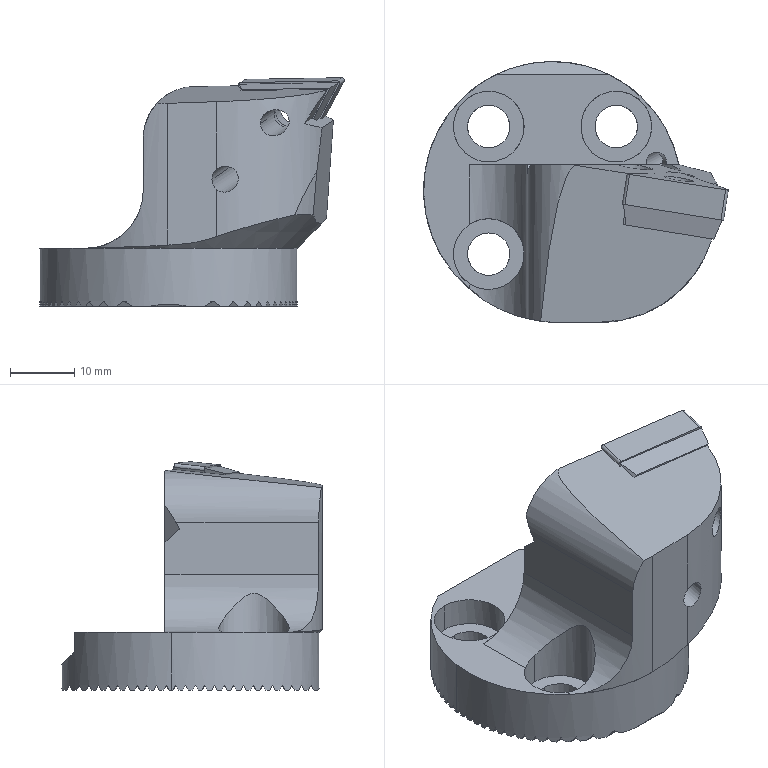CAM job | Mastercam | 3-axis milling, 5-axis milling, drilling
Tools:
tool_number,name,type,diameter_mm,corner_radius_mm,flutes,flute_length_mm,overall_length_mm,shoulder_length_mm,holder_diameter_mm,length_offset,diameter_offset,default_rpm,default_feed_mm_min,default_plunge_mm_min,coolant
1,1.6 Drill,drill,1.6,0,2,10,15,10,16.002,1,1,3750,450,600,COOL_OFF
2,5 Chamfer Mill,chamfer mill,5,0,4,25,25,25,31.877,2,2,5000,600,600,COOL_OFF
3,6 Drill,drill,6,0,2,25,30,25,27.495,3,3,1000,120.0,600,COOL_OFF
4,12 Flat End Mill Rough,end mill,12,0,4,30,30,30,42.012,4,4,833,99.96,600,COOL_OFF
5,6 Flat End Mill Rough,end mill,6,0,4,25,25,25,31.877,5,5,1667,200.04,600,COOL_OFF
6,4 Flat End Mill Rough,end mill,4,0,4,25,25,25,27.495,6,6,2500,300,600,COOL_OFF
7,4 Flat End Mill Finish,end mill,4,0,4,25,25,25,27.495,7,7,2500,300,600,COOL_OFF
8,2 Taper Mill,tap,2,0,4,16.29,30,16.29,31.877,8,8,3000,360,600,COOL_OFF
9,12 Flat End Mill Finish,end mill,12,0,4,30,30,30,42.012,9,9,833,99.96,600,COOL_OFF
10,30 Insert Cutter,bull end mill,30,0.8,4,25,60,25,47.625,10,10,400,48.0,600,COOL_OFF
11,4.5 Flat End Mill,end mill,4.5,0,4,20,20,20,31.877,11,11,2222,266.64,600,COOL_OFF
12,6 Chamfer Mill,chamfer mill,6,0,4,25,25,25,31.877,12,12,4167,500.04,600,COOL_OFF
13,3.3 Drill,drill,3.3,0,2,25,38,35,31.877,13,13,1818,218.16,600,COOL_OFF
14,M4 3-tooth Thread Mill,thread mill,3.15,0,4,2.1,20,2.1,31.877,14,14,1905,228.6,600,COOL_OFF
15,2.5 Ball Mill,ball end mill,2.5,1.25,4,4,20,4,31.877,15,15,4800,576,600,COOL_OFF
16,M4 x 0.7 RH Tap,drill,4,0,2,20,23,20,31.877,16,16,1500,1050,600,COOL_OFF
17,2.9 Drill,drill,2.9,0,2,25,35,25,31.877,17,17,2069,248.28,600,COOL_OFF
18,8 Flat End Mill,end mill,8,0,4,25,25,25,31.877,18,18,1250,150,600,COOL_OFF
Operations:
seq,operation,operation_type,tool_number,tool_name,tool_diameter_mm,spindle_rpm,feed_mm_min,plunge_mm_min,retract_mm_min,cycle_time_s,wcs,posted,nc_file
1,Contour (2D) - [WCS: Top] - [Tplane: Out],Contour,18,8 Flat End Mill,8,3500,1500,2000,1200,19.605,Top,yes,1.nc
2,Drill/Counterbore - [WCS: Top] - [Tplane: Out],Drill,2,5 Chamfer Mill,5,2000,100,600,1200,1.643,Top,yes,1.nc
3,Drill/Counterbore - [WCS: Top] - [Tplane: M4Pl],Drill,2,5 Chamfer Mill,5,2000,100,600,1200,1.934,Top,yes,1.nc
4,Peck Drill - [WCS: Top] - [Tplane: M4Pl],Drill,13,3.3 Drill,3.3,3000,60,600,1200,23.325,Top,yes,1.nc
5,Peck Drill - [WCS: Top] - [Tplane: Out],Drill,17,2.9 Drill,2.9,3000,60,600,1200,27.431,Top,yes,1.nc
6,2D High Speed (2D Dynamic Mill) - [WCS: Top] - [Tplane: Top],HighSpeed2D,4,12 Flat End Mill Rough,12,3500,2500,2000,1200,39.474,Top,yes,1.nc
7,2D High Speed (2D Dynamic Mill) - [WCS: Top] - [Tplane: A90],HighSpeed2D,4,12 Flat End Mill Rough,12,3500,2000,2000,1200,236.176,Top,yes,1.nc
8,Contour (2D) - [WCS: Top] - [Tplane: In],Contour,4,12 Flat End Mill Rough,12,3500,2000,2000,1200,6.585,Top,yes,1.nc
9,Contour (2D) - [WCS: Top] - [Tplane: A90],Contour,4,12 Flat End Mill Rough,12,3500,2000,2000,1200,2.545,Top,yes,1.nc
10,Contour (Ramp) - [WCS: Top] - [Tplane: A90],Contour,4,12 Flat End Mill Rough,12,3500,2000,2000,1200,5.869,Top,yes,1.nc
11,2D High Speed (2D Dynamic Mill) - [WCS: Top] - [Tplane: A90-1],HighSpeed2D,4,12 Flat End Mill Rough,12,3500,2000,2000,1200,131.829,Top,yes,1.nc
12,Contour (2D) - [WCS: Top] - [Tplane: In],Contour,4,12 Flat End Mill Rough,12,3500,1000,2000,1200,19.432,Top,yes,1.nc
13,Contour (Ramp) - [WCS: Top] - [Tplane: A45],Contour,4,12 Flat End Mill Rough,12,3500,2000,2000,1200,2.522,Top,yes,1.nc
14,Contour (2D) - [WCS: Top] - [Tplane: 4],Contour,4,12 Flat End Mill Rough,12,3500,2000,2000,1200,8.359,Top,yes,1.nc
15,Contour (2D) - [WCS: Top] - [Tplane: 6],Contour,4,12 Flat End Mill Rough,12,3500,2000,2000,1200,5.429,Top,yes,1.nc
16,2D High Speed (2D Dynamic Mill) - [WCS: Top] - [Tplane: In],HighSpeed2D,5,6 Flat End Mill Rough,6,3500,1500,2000,1200,34.984,Top,yes,1.nc
17,Contour (2D) - [WCS: Top] - [Tplane: In],Contour,6,4 Flat End Mill Rough,4,3500,500,2000,1200,101.062,Top,yes,1.nc
18,Contour (2D) - [WCS: Top] - [Tplane: In],Contour,6,4 Flat End Mill Rough,4,3500,500,2000,1200,4.18,Top,yes,1.nc
19,Contour (2D) - [WCS: Top] - [Tplane: Top],Contour,9,12 Flat End Mill Finish,12,3500,600,2000,1200,8.36,Top,yes,1.nc
20,Contour (2D) - [WCS: Top] - [Tplane: A90],Contour,9,12 Flat End Mill Finish,12,3500,600,2000,1200,7.305,Top,yes,1.nc
21,Contour (2D) - [WCS: Top] - [Tplane: A90],Contour,9,12 Flat End Mill Finish,12,3500,600,2000,1200,4.049,Top,yes,1.nc
22,Contour (2D) - [WCS: Top] - [Tplane: In],Contour,9,12 Flat End Mill Finish,12,3500,600,2000,1200,3.402,Top,yes,1.nc
23,Contour (2D) - [WCS: Top] - [Tplane: A90-1],Contour,9,12 Flat End Mill Finish,12,3500,600,2000,1200,8.595,Top,yes,1.nc
24,Contour (2D) - [WCS: Top] - [Tplane: In],Contour,9,12 Flat End Mill Finish,12,3500,600,2000,1200,4.652,Top,yes,1.nc
25,Contour (2D) - [WCS: Top] - [Tplane: A45],Contour,9,12 Flat End Mill Finish,12,3500,600,2000,1200,3.943,Top,yes,1.nc
26,Contour (2D) - [WCS: Top] - [Tplane: 6],Contour,9,12 Flat End Mill Finish,12,3500,600,2000,1200,3.218,Top,yes,1.nc
27,Contour (2D) - [WCS: Top] - [Tplane: A90],Contour,10,30 Insert Cutter,30,3500,400,2000,1200,13.44,Top,yes,1.nc
28,Contour (2D) - [WCS: Top] - [Tplane: In],Contour,10,30 Insert Cutter,30,3500,600,2000,1200,6.789,Top,yes,1.nc
29,Drill/Counterbore - [WCS: Top] - [Tplane: In],Drill,12,6 Chamfer Mill,6,2000,100,600,1200,4.705,Top,yes,1.nc
30,Drill/Counterbore - [WCS: Top] - [Tplane: In],Drill,3,6 Drill,6,2500,100,600,1200,4.574,Top,yes,1.nc
31,Peck Drill - [WCS: Top] - [Tplane: In],Drill,13,3.3 Drill,3.3,2500,60,600,1200,14.924,Top,yes,1.nc
32,Peck Drill - [WCS: Top] - [Tplane: In],Drill,13,3.3 Drill,3.3,2500,60,600,1200,27.051,Top,yes,1.nc
33,Manual Entry (M0),ManualEntry,,,,0,0,0,0,0,Top,yes,1.nc
34,Drill/Counterbore - [WCS: Top] - [Tplane: In],Drill,12,6 Chamfer Mill,6,2000,100,600,1200,2.397,Top,yes,1.nc
35,Drill/Counterbore - [WCS: Top] - [Tplane: CB],Drill,11,4.5 Flat End Mill,4.5,2000,100,600,1200,4.09,Top,yes,1.nc
36,Peck Drill - [WCS: Top] - [Tplane: CB],Drill,11,4.5 Flat End Mill,4.5,2000,100,600,1200,7.397,Top,yes,1.nc
37,Thread Mill - [WCS: Top] - [Tplane: In],ThreadMill,14,M4 3-tooth Thread Mill,3.15,2500,100,600,1200,43.422,Top,yes,1.nc
38,Thread Mill - [WCS: Top] - [Tplane: M4Pl],ThreadMill,14,M4 3-tooth Thread Mill,3.15,2500,100,600,1200,21.533,Top,yes,1.nc
39,Tap - [WCS: Top] - [Tplane: In],Drill,16,M4 x 0.7 RH Tap,4,300,210.0,600,1200,17.66,Top,yes,1.nc
40,Peck Drill - [WCS: Top] - [Tplane: In],Drill,1,1.6 Drill,1.6,3000,60,600,1200,6.789,Top,yes,1.nc
41,Stock model - [WCS: Top] - [Tplane: Top] - 1,139,,,,0,0,0,0,0,Top,yes,1.nc
42,Contour (2D) - [WCS: Top] - [Tplane: Pl],Contour,5,6 Flat End Mill Rough,6,3500,800,2000,1200,43.427,Top,yes,1.nc
43,Contour (Remachining) - [WCS: Top] - [Tplane: Pl],Contour,6,4 Flat End Mill Rough,4,3500,600,2000,1200,11.577,Top,yes,1.nc
44,Circle Mill - [WCS: Top] - [Tplane: In],CircleMill,6,4 Flat End Mill Rough,4,3500,200,2000,3.581,11.514,Top,yes,1.nc
45,Contour (2D) - [WCS: Top] - [Tplane: Pl],Contour,7,4 Flat End Mill Finish,4,3500,400,2000,1200,9.203,Top,yes,1.nc
46,Contour (2D) - [WCS: Top] - [Tplane: Pl-5],Contour,7,4 Flat End Mill Finish,4,3500,400,2000,1200,3.516,Top,yes,1.nc
47,Contour (2D) - [WCS: Top] - [Tplane: Pl-6],Contour,7,4 Flat End Mill Finish,4,3500,400,2000,1200,5.527,Top,yes,1.nc
48,Contour (2D) - [WCS: Top] - [Tplane: In],Contour,7,4 Flat End Mill Finish,4,3500,400,2000,1200,9.27,Top,yes,1.nc
49,Contour (2D) - [WCS: Top] - [Tplane: In],Contour,7,4 Flat End Mill Finish,4,3500,400,2000,1200,9.981,Top,yes,1.nc
50,Contour (2D) - [WCS: Top] - [Tplane: In],Contour,7,4 Flat End Mill Finish,4,3500,400,2000,1200,9.981,Top,yes,1.nc
51,Deburr 5-axis - [WCS: Top] - [Tplane: Top],459,15,2.5 Ball Mill,2.5,4500,1000,2000,3.581,10.199,Top,yes,1.nc
52,Deburr 5-axis - [WCS: Top] - [Tplane: Top],459,15,2.5 Ball Mill,2.5,4500,1000,2000,3.581,4.955,Top,yes,1.nc
53,Swarf machining - [WCS: Top] - [Tplane: Top],441,7,4 Flat End Mill Finish,4,2500,300,600,1200,7.29,Top,yes,2.nc
54,Contour (2D) - [WCS: Top] - [Tplane: Pl-5],Contour,7,4 Flat End Mill Finish,4,3500,400,2000,1200,3.516,Top,yes,3.nc
55,Contour (2D) - [WCS: Top] - [Tplane: Pl-6],Contour,7,4 Flat End Mill Finish,4,3500,400,2000,1200,5.527,Top,yes,3.nc